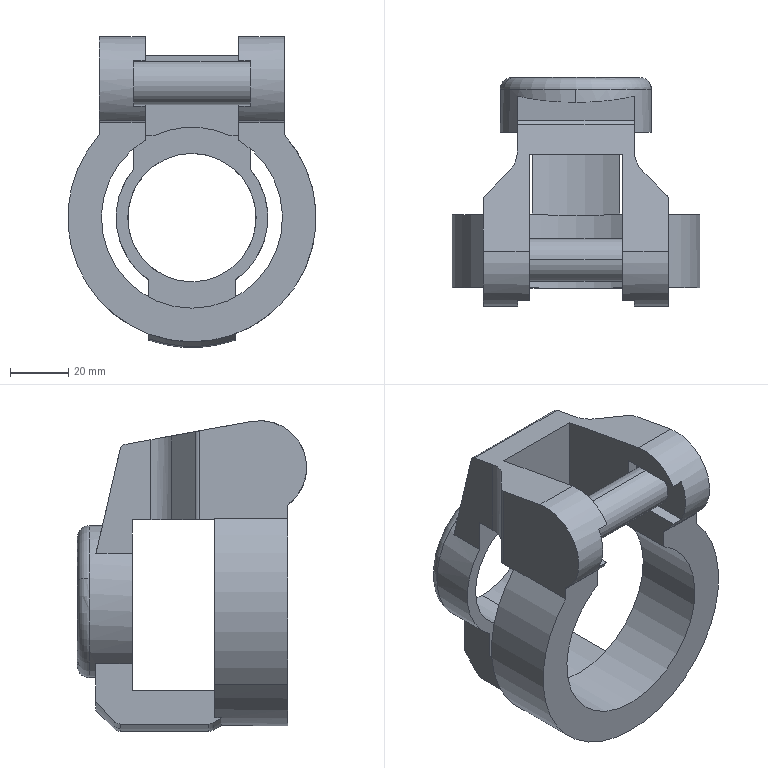Part | NX | features BREP 1 | 1 solid | 54 faces | box 85 x 78.5 x 106.5 mm | volume 141496 mm3 | plane 27 | cylinder 21 | torus 4 | cone 2 | commonest cylinder face diameters 4 x3 2 x2 14.75 x2 20 x2 32 x2 44 x2